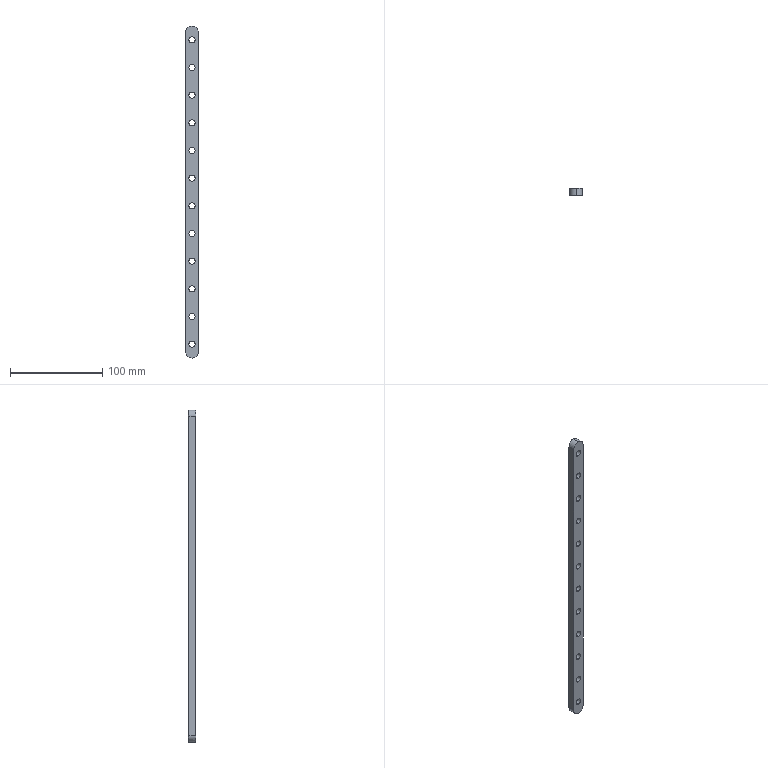Part | SolidWorks | features ICE 2, Extrusion 1, Fillet 1, HoleWzd 1, LPattern 1 | 1 solid | 70 faces | box 14 x 8 x 360 mm | volume 35757 mm3 | cylinder 28 | cone 24 | plane 18 | commonest cylinder face diameters 6.8 x24 14 x4